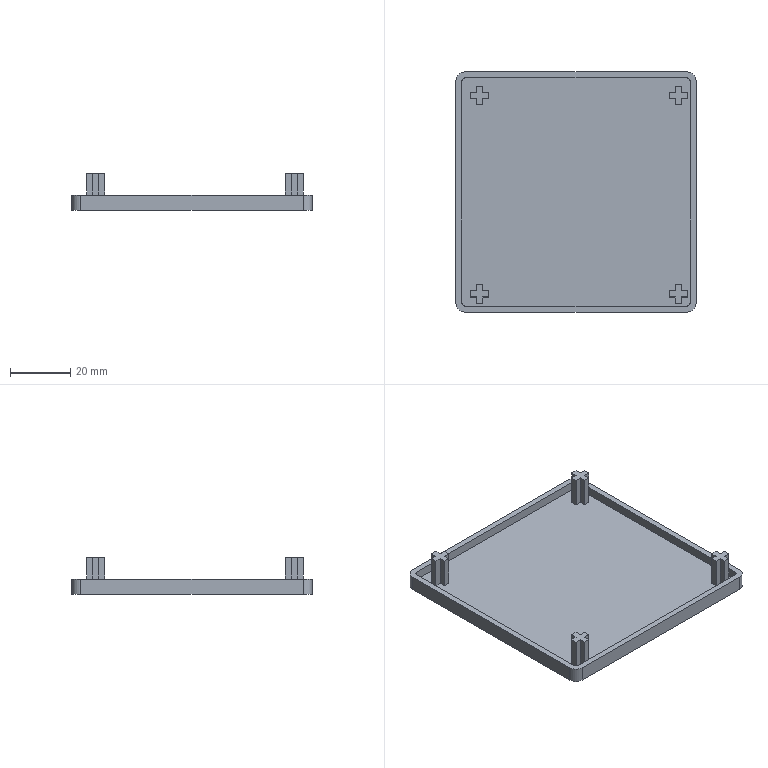Part | NX | 1 solid | 71 faces | box 80 x 80 x 12 mm | volume 15436 mm3 | plane 63 | cylinder 8 | commonest cylinder face diameters 2 x4 6 x4